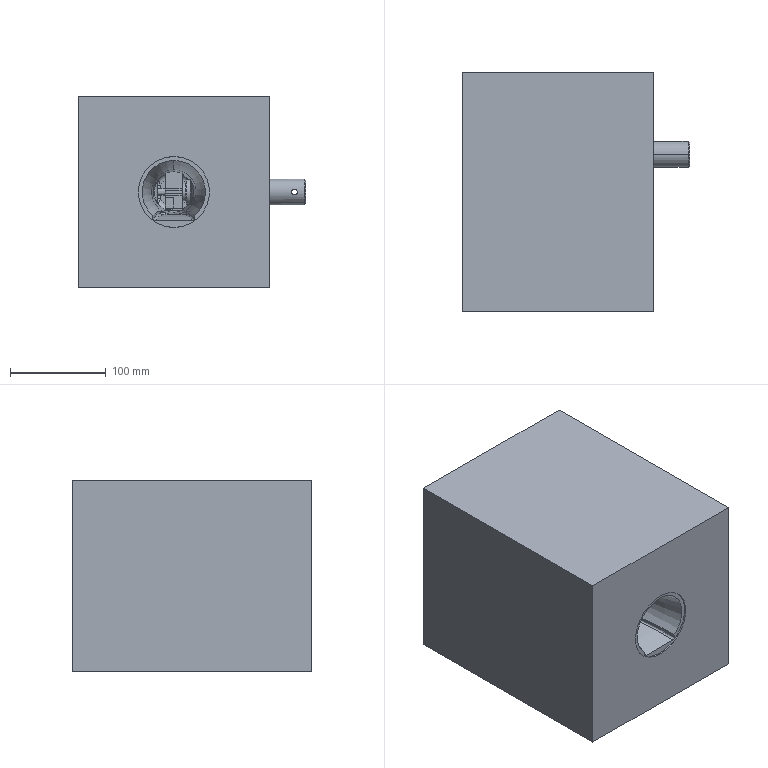Part | STEP file | Cavity - Tower - 1 cav - Insert 1 | 2 solids | 111 faces | box 238 x 250 x 200 mm | volume 9730114 mm3 | plane 44 | spline 24 | cylinder 17 | cone 15 | torus 9 | sphere 2 | commonest cylinder face diameters 27 x6 1.018 x2 6 x2 6.105 x2 20.711 x2 28.622 x2